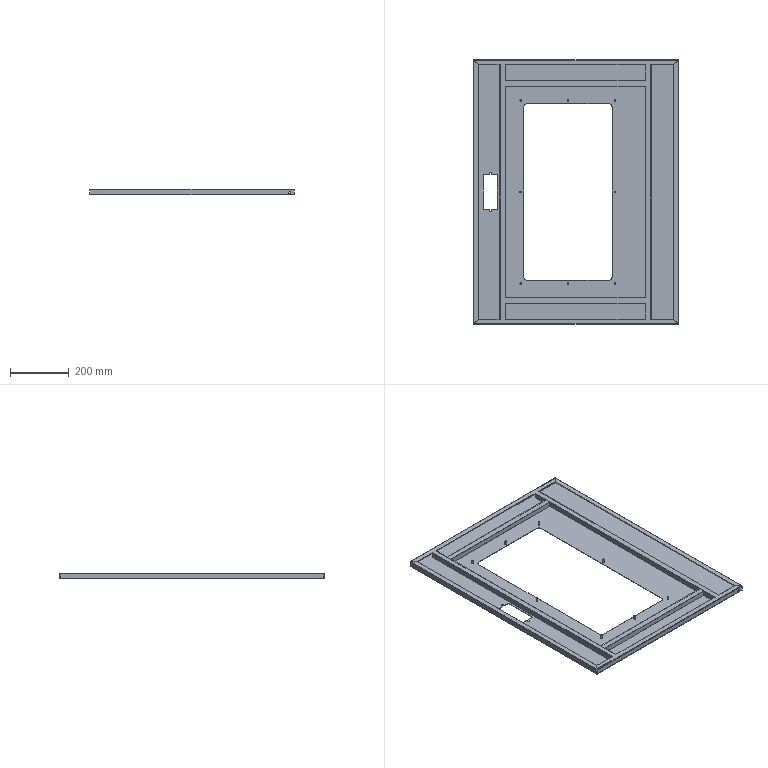Part | STEP file | MB-005 | 1 solid | 152 faces | box 700 x 900 x 20 mm | volume 1064714 mm3 | plane 92 | cylinder 44 | spline 16 | commonest cylinder face diameters 6 x20 1.473 x8 4.473 x8 20 x4 4 x2 7 x2